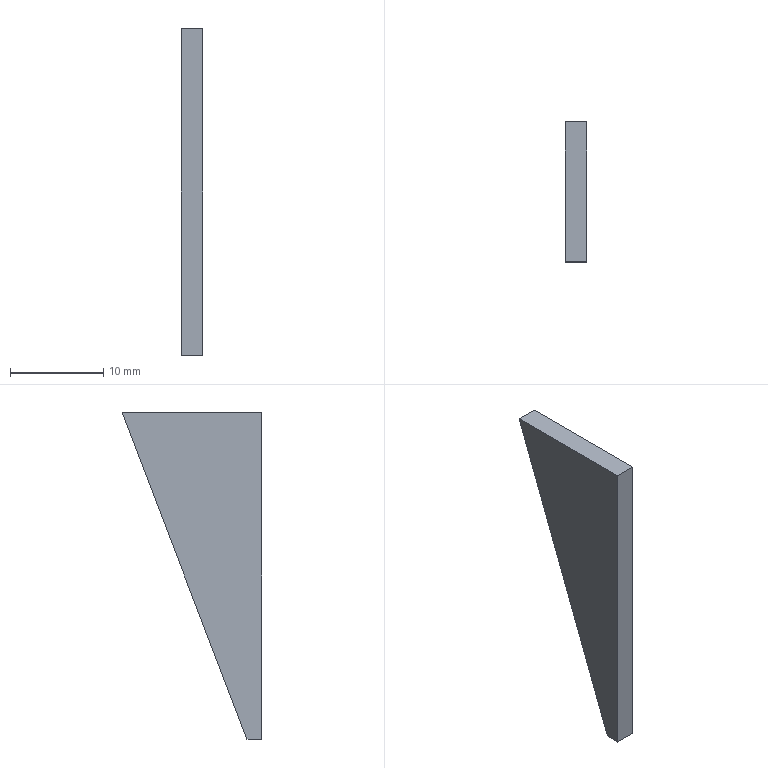Part | SolidWorks | features FlatPattern 1, SMBaseFlange 1, SheetMetal 1 | 1 solid | 6 faces | box 2.3 x 15 x 35 mm | volume 668.15 mm3 | plane 6
STEP:
#1=CARTESIAN_POINT('',(0.,15.,0.));
#2=VERTEX_POINT('',#1);
#3=CARTESIAN_POINT('',(0.,0.,0.));
#4=VERTEX_POINT('',#3);
#5=CARTESIAN_POINT('',(0.,15.,0.));
#6=DIRECTION('',(0.,-1.,0.));
#7=VECTOR('',#6,1000.);
#8=LINE('',#5,#7);
#9=EDGE_CURVE('',#2,#4,#8,.T.);
#10=ORIENTED_EDGE('',*,*,#9,.F.);
#11=CARTESIAN_POINT('',(-2.3,15.,0.));
#12=VERTEX_POINT('',#11);
#13=CARTESIAN_POINT('',(-2.3,15.,0.));
#14=DIRECTION('',(1.,0.,0.));
#15=VECTOR('',#14,1000.);
#16=LINE('',#13,#15);
#17=EDGE_CURVE('',#12,#2,#16,.T.);
#18=ORIENTED_EDGE('',*,*,#17,.F.);
#19=CARTESIAN_POINT('',(-2.3,0.,0.));
#20=VERTEX_POINT('',#19);
#21=CARTESIAN_POINT('',(-2.3,15.,0.));
#22=DIRECTION('',(0.,-1.,0.));
#23=VECTOR('',#22,1000.);
#24=LINE('',#21,#23);
#25=EDGE_CURVE('',#12,#20,#24,.T.);
#26=ORIENTED_EDGE('',*,*,#25,.T.);
#27=CARTESIAN_POINT('',(-2.3,0.,0.));
#28=DIRECTION('',(1.,0.,0.));
#29=VECTOR('',#28,1000.);
#30=LINE('',#27,#29);
#31=EDGE_CURVE('',#20,#4,#30,.T.);
#32=ORIENTED_EDGE('',*,*,#31,.T.);
#33=EDGE_LOOP('',(#10,#18,#26,#32));
#34=FACE_OUTER_BOUND('',#33,.T.);
#35=CARTESIAN_POINT('',(-2.3,15.,0.));
#36=DIRECTION('',(0.,0.,1.));
#37=DIRECTION('',(0.,-1.,0.));
#38=AXIS2_PLACEMENT_3D('',#35,#36,#37);
#39=PLANE('',#38);
#40=ADVANCED_FACE('',(#34),#39,.T.);
#41=CARTESIAN_POINT('',(0.,1.6,-35.));
#42=VERTEX_POINT('',#41);
#43=CARTESIAN_POINT('',(0.,1.6,-35.));
#44=DIRECTION('',(0.,0.3575,0.9339));
#45=VECTOR('',#44,1000.);
#46=LINE('',#43,#45);
#47=EDGE_CURVE('',#42,#2,#46,.T.);
#48=ORIENTED_EDGE('',*,*,#47,.F.);
#49=CARTESIAN_POINT('',(-2.3,1.6,-35.));
#50=VERTEX_POINT('',#49);
#51=CARTESIAN_POINT('',(-2.3,1.6,-35.));
#52=DIRECTION('',(1.,0.,0.));
#53=VECTOR('',#52,1000.);
#54=LINE('',#51,#53);
#55=EDGE_CURVE('',#50,#42,#54,.T.);
#56=ORIENTED_EDGE('',*,*,#55,.F.);
#57=CARTESIAN_POINT('',(-2.3,1.6,-35.));
#58=DIRECTION('',(0.,0.3575,0.9339));
#59=VECTOR('',#58,1000.);
#60=LINE('',#57,#59);
#61=EDGE_CURVE('',#50,#12,#60,.T.);
#62=ORIENTED_EDGE('',*,*,#61,.T.);
#63=ORIENTED_EDGE('',*,*,#17,.T.);
#64=EDGE_LOOP('',(#48,#56,#62,#63));
#65=FACE_OUTER_BOUND('',#64,.T.);
#66=CARTESIAN_POINT('',(-2.3,1.6,-35.));
#67=DIRECTION('',(0.,0.9339,-0.3575));
#68=DIRECTION('',(0.,0.3575,0.9339));
#69=AXIS2_PLACEMENT_3D('',#66,#67,#68);
#70=PLANE('',#69);
#71=ADVANCED_FACE('',(#65),#70,.T.);
#72=CARTESIAN_POINT('',(0.,0.,-35.));
#73=VERTEX_POINT('',#72);
#74=CARTESIAN_POINT('',(0.,0.,-35.));
#75=DIRECTION('',(0.,1.,0.));
#76=VECTOR('',#75,1000.);
#77=LINE('',#74,#76);
#78=EDGE_CURVE('',#73,#42,#77,.T.);
#79=ORIENTED_EDGE('',*,*,#78,.F.);
#80=CARTESIAN_POINT('',(-2.3,0.,-35.));
#81=VERTEX_POINT('',#80);
#82=CARTESIAN_POINT('',(-2.3,0.,-35.));
#83=DIRECTION('',(1.,0.,0.));
#84=VECTOR('',#83,1000.);
#85=LINE('',#82,#84);
#86=EDGE_CURVE('',#81,#73,#85,.T.);
#87=ORIENTED_EDGE('',*,*,#86,.F.);
#88=CARTESIAN_POINT('',(-2.3,0.,-35.));
#89=DIRECTION('',(0.,1.,0.));
#90=VECTOR('',#89,1000.);
#91=LINE('',#88,#90);
#92=EDGE_CURVE('',#81,#50,#91,.T.);
#93=ORIENTED_EDGE('',*,*,#92,.T.);
#94=ORIENTED_EDGE('',*,*,#55,.T.);
#95=EDGE_LOOP('',(#79,#87,#93,#94));
#96=FACE_OUTER_BOUND('',#95,.T.);
#97=CARTESIAN_POINT('',(-2.3,0.,-35.));
#98=DIRECTION('',(0.,0.,-1.));
#99=DIRECTION('',(-1.,0.,0.));
#100=AXIS2_PLACEMENT_3D('',#97,#98,#99);
#101=PLANE('',#100);
#102=ADVANCED_FACE('',(#96),#101,.T.);
#103=CARTESIAN_POINT('',(0.,0.,0.));
#104=DIRECTION('',(0.,0.,-1.));
#105=VECTOR('',#104,1000.);
#106=LINE('',#103,#105);
#107=EDGE_CURVE('',#4,#73,#106,.T.);
#108=ORIENTED_EDGE('',*,*,#107,.F.);
#109=ORIENTED_EDGE('',*,*,#31,.F.);
#110=CARTESIAN_POINT('',(-2.3,0.,0.));
#111=DIRECTION('',(0.,0.,-1.));
#112=VECTOR('',#111,1000.);
#113=LINE('',#110,#112);
#114=EDGE_CURVE('',#20,#81,#113,.T.);
#115=ORIENTED_EDGE('',*,*,#114,.T.);
#116=ORIENTED_EDGE('',*,*,#86,.T.);
#117=EDGE_LOOP('',(#108,#109,#115,#116));
#118=FACE_OUTER_BOUND('',#117,.T.);
#119=CARTESIAN_POINT('',(-2.3,0.,0.));
#120=DIRECTION('',(0.,-1.,0.));
#121=DIRECTION('',(0.,0.,-1.));
#122=AXIS2_PLACEMENT_3D('',#119,#120,#121);
#123=PLANE('',#122);
#124=ADVANCED_FACE('',(#118),#123,.T.);
#125=ORIENTED_EDGE('',*,*,#25,.F.);
#126=ORIENTED_EDGE('',*,*,#61,.F.);
#127=ORIENTED_EDGE('',*,*,#92,.F.);
#128=ORIENTED_EDGE('',*,*,#114,.F.);
#129=EDGE_LOOP('',(#125,#126,#127,#128));
#130=FACE_OUTER_BOUND('',#129,.T.);
#131=CARTESIAN_POINT('',(-2.3,0.,0.));
#132=DIRECTION('',(1.,0.,0.));
#133=DIRECTION('',(0.,0.,-1.));
#134=AXIS2_PLACEMENT_3D('',#131,#132,#133);
#135=PLANE('',#134);
#136=ADVANCED_FACE('',(#130),#135,.F.);
#137=ORIENTED_EDGE('',*,*,#9,.T.);
#138=ORIENTED_EDGE('',*,*,#107,.T.);
#139=ORIENTED_EDGE('',*,*,#78,.T.);
#140=ORIENTED_EDGE('',*,*,#47,.T.);
#141=EDGE_LOOP('',(#137,#138,#139,#140));
#142=FACE_OUTER_BOUND('',#141,.T.);
#143=CARTESIAN_POINT('',(0.,0.,0.));
#144=DIRECTION('',(1.,0.,0.));
#145=DIRECTION('',(0.,0.,-1.));
#146=AXIS2_PLACEMENT_3D('',#143,#144,#145);
#147=PLANE('',#146);
#148=ADVANCED_FACE('',(#142),#147,.T.);
#149=CLOSED_SHELL('',(#40,#71,#102,#124,#136,#148));
#150=MANIFOLD_SOLID_BREP('',#149);
#151=CARTESIAN_POINT('',(0.,0.,0.));
#152=DIRECTION('',(0.,0.,1.));
#153=DIRECTION('',(1.,0.,0.));
#154=AXIS2_PLACEMENT_3D('',#151,#152,#153);
#155=(LENGTH_UNIT()NAMED_UNIT(*)SI_UNIT(.MILLI.,.METRE.));
#156=UNCERTAINTY_MEASURE_WITH_UNIT(LENGTH_MEASURE(0.00001),#155,'','');
#157=(NAMED_UNIT(*)PLANE_ANGLE_UNIT()SI_UNIT($,.RADIAN.));
#158=(NAMED_UNIT(*)SI_UNIT($,.STERADIAN.)SOLID_ANGLE_UNIT());
#159=(GEOMETRIC_REPRESENTATION_CONTEXT(3)GLOBAL_UNCERTAINTY_ASSIGNED_CONTEXT((#156))GLOBAL_UNIT_ASSIGNED_CONTEXT((#155,#157,#158))REPRESENTATION_CONTEXT('',''));
#160=ADVANCED_BREP_SHAPE_REPRESENTATION('',(#150,#154),#159);